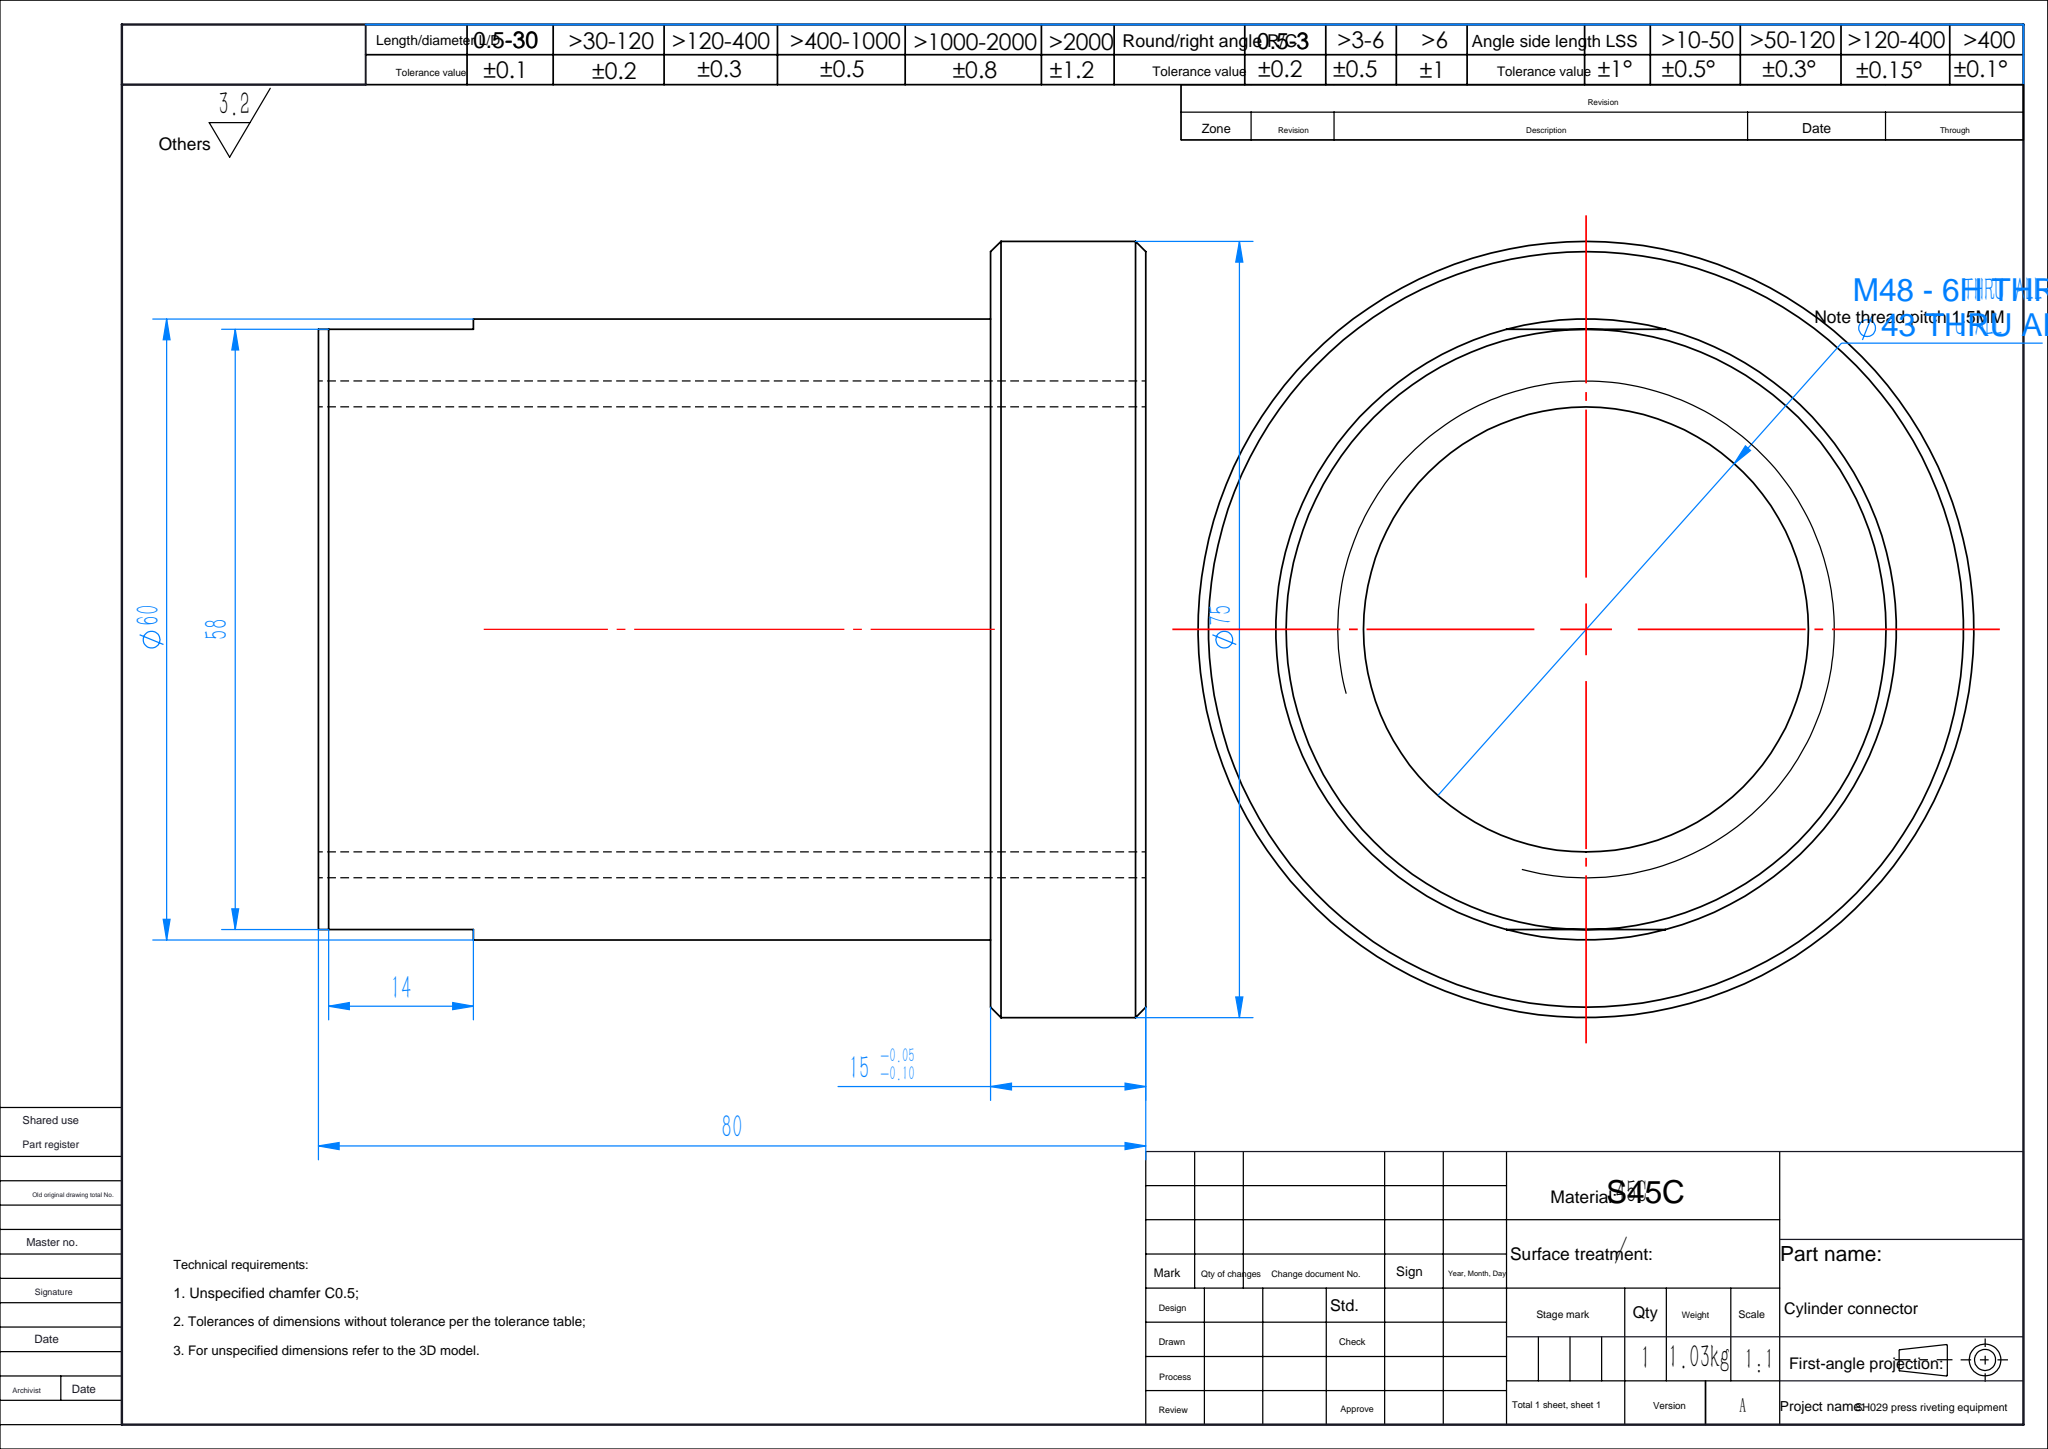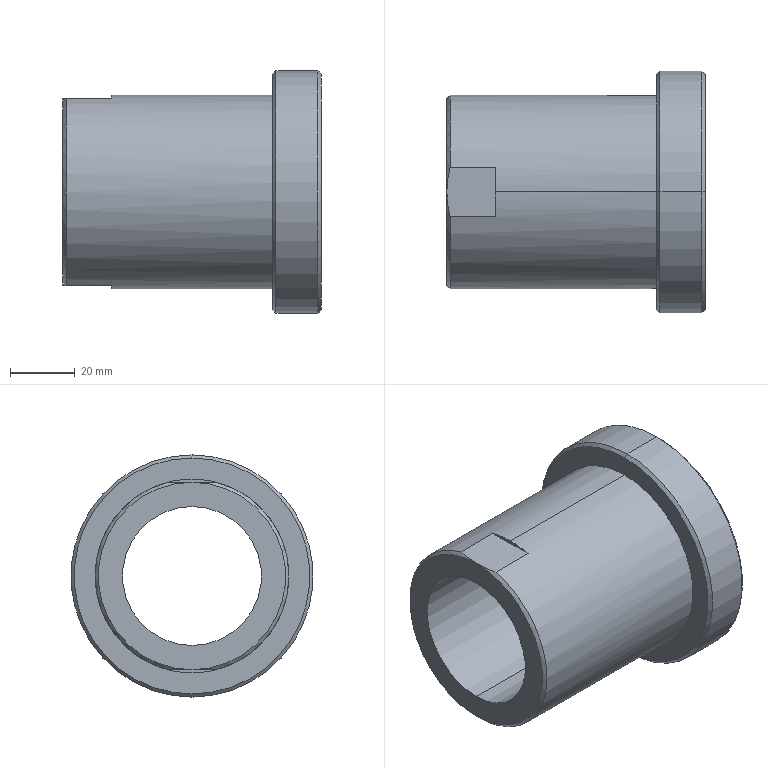Part | SolidWorks | features Chamfer 1, HoleWzd 1, ICE 1, LibraryFeature 1, Revolution 1 | 1 solid | 19 faces | box 80 x 75 x 75 mm | volume 133252 mm3 | plane 7 | cone 6 | cylinder 6 | commonest cylinder face diameters 43 x2 60 x2 75 x2
STEP:
#1=CARTESIAN_POINT('',(25.,0.,36.5));
#2=VERTEX_POINT('',#1);
#3=CARTESIAN_POINT('',(25.,0.,-36.5));
#4=VERTEX_POINT('',#3);
#5=CARTESIAN_POINT('',(25.,0.,0.));
#6=DIRECTION('',(-1.,0.,0.));
#7=DIRECTION('',(0.,0.,-1.));
#8=AXIS2_PLACEMENT_3D('',#5,#6,#7);
#9=CIRCLE('',#8,36.5);
#10=EDGE_CURVE('',#2,#4,#9,.T.);
#11=ORIENTED_EDGE('',*,*,#10,.F.);
#12=CARTESIAN_POINT('',(26.,0.,37.5));
#13=VERTEX_POINT('',#12);
#14=CARTESIAN_POINT('',(25.,0.,36.5));
#15=DIRECTION('',(0.7071,0.,0.7071));
#16=VECTOR('',#15,1000.);
#17=LINE('',#14,#16);
#18=EDGE_CURVE('',#2,#13,#17,.T.);
#19=ORIENTED_EDGE('',*,*,#18,.T.);
#20=CARTESIAN_POINT('',(26.,0.,-37.5));
#21=VERTEX_POINT('',#20);
#22=CARTESIAN_POINT('',(26.,0.,0.));
#23=DIRECTION('',(1.,0.,0.));
#24=DIRECTION('',(0.,0.,-1.));
#25=AXIS2_PLACEMENT_3D('',#22,#23,#24);
#26=CIRCLE('',#25,37.5);
#27=EDGE_CURVE('',#21,#13,#26,.T.);
#28=ORIENTED_EDGE('',*,*,#27,.F.);
#29=CARTESIAN_POINT('',(25.,0.,-36.5));
#30=DIRECTION('',(0.7071,0.,-0.7071));
#31=VECTOR('',#30,1000.);
#32=LINE('',#29,#31);
#33=EDGE_CURVE('',#4,#21,#32,.T.);
#34=ORIENTED_EDGE('',*,*,#33,.F.);
#35=EDGE_LOOP('',(#11,#19,#28,#34));
#36=FACE_OUTER_BOUND('',#35,.T.);
#37=CARTESIAN_POINT('',(25.,0.,0.));
#38=DIRECTION('',(1.,0.,0.));
#39=DIRECTION('',(0.,0.,-1.));
#40=AXIS2_PLACEMENT_3D('',#37,#38,#39);
#41=CONICAL_SURFACE('',#40,36.5,0.7854);
#42=ADVANCED_FACE('',(#36),#41,.T.);
#43=CARTESIAN_POINT('',(40.,0.,-36.5));
#44=VERTEX_POINT('',#43);
#45=CARTESIAN_POINT('',(40.,0.,36.5));
#46=VERTEX_POINT('',#45);
#47=CARTESIAN_POINT('',(40.,0.,0.));
#48=DIRECTION('',(1.,0.,0.));
#49=DIRECTION('',(0.,0.,1.));
#50=AXIS2_PLACEMENT_3D('',#47,#48,#49);
#51=CIRCLE('',#50,36.5);
#52=EDGE_CURVE('',#44,#46,#51,.T.);
#53=ORIENTED_EDGE('',*,*,#52,.F.);
#54=CARTESIAN_POINT('',(39.,0.,-37.5));
#55=VERTEX_POINT('',#54);
#56=CARTESIAN_POINT('',(39.,0.,-37.5));
#57=DIRECTION('',(-0.7071,0.,-0.7071));
#58=VECTOR('',#57,1000.);
#59=LINE('',#56,#58);
#60=EDGE_CURVE('',#44,#55,#59,.T.);
#61=ORIENTED_EDGE('',*,*,#60,.T.);
#62=CARTESIAN_POINT('',(39.,0.,37.5));
#63=VERTEX_POINT('',#62);
#64=CARTESIAN_POINT('',(39.,0.,0.));
#65=DIRECTION('',(-1.,0.,0.));
#66=DIRECTION('',(0.,0.,1.));
#67=AXIS2_PLACEMENT_3D('',#64,#65,#66);
#68=CIRCLE('',#67,37.5);
#69=EDGE_CURVE('',#63,#55,#68,.T.);
#70=ORIENTED_EDGE('',*,*,#69,.F.);
#71=CARTESIAN_POINT('',(39.,0.,37.5));
#72=DIRECTION('',(-0.7071,0.,0.7071));
#73=VECTOR('',#72,1000.);
#74=LINE('',#71,#73);
#75=EDGE_CURVE('',#46,#63,#74,.T.);
#76=ORIENTED_EDGE('',*,*,#75,.F.);
#77=EDGE_LOOP('',(#53,#61,#70,#76));
#78=FACE_OUTER_BOUND('',#77,.T.);
#79=CARTESIAN_POINT('',(39.,0.,0.));
#80=DIRECTION('',(-1.,0.,0.));
#81=DIRECTION('',(0.,0.,1.));
#82=AXIS2_PLACEMENT_3D('',#79,#80,#81);
#83=CONICAL_SURFACE('',#82,37.5,0.7854);
#84=ADVANCED_FACE('',(#78),#83,.T.);
#85=CARTESIAN_POINT('',(40.,0.,-21.5));
#86=VERTEX_POINT('',#85);
#87=CARTESIAN_POINT('',(40.,0.,21.5));
#88=VERTEX_POINT('',#87);
#89=CARTESIAN_POINT('',(40.,0.,0.));
#90=DIRECTION('',(-1.,0.,0.));
#91=DIRECTION('',(0.,0.,1.));
#92=AXIS2_PLACEMENT_3D('',#89,#90,#91);
#93=CIRCLE('',#92,21.5);
#94=EDGE_CURVE('',#86,#88,#93,.T.);
#95=ORIENTED_EDGE('',*,*,#94,.F.);
#96=CARTESIAN_POINT('',(-40.,0.,-21.5));
#97=VERTEX_POINT('',#96);
#98=CARTESIAN_POINT('',(-40.,0.,-21.5));
#99=DIRECTION('',(-1.,0.,0.));
#100=VECTOR('',#99,1000.);
#101=LINE('',#98,#100);
#102=EDGE_CURVE('',#86,#97,#101,.T.);
#103=ORIENTED_EDGE('',*,*,#102,.T.);
#104=CARTESIAN_POINT('',(-40.,0.,21.5));
#105=VERTEX_POINT('',#104);
#106=CARTESIAN_POINT('',(-40.,0.,0.));
#107=DIRECTION('',(-1.,0.,0.));
#108=DIRECTION('',(0.,0.,1.));
#109=AXIS2_PLACEMENT_3D('',#106,#107,#108);
#110=CIRCLE('',#109,21.5);
#111=EDGE_CURVE('',#97,#105,#110,.T.);
#112=ORIENTED_EDGE('',*,*,#111,.T.);
#113=CARTESIAN_POINT('',(-40.,0.,21.5));
#114=DIRECTION('',(-1.,0.,0.));
#115=VECTOR('',#114,1000.);
#116=LINE('',#113,#115);
#117=EDGE_CURVE('',#88,#105,#116,.T.);
#118=ORIENTED_EDGE('',*,*,#117,.F.);
#119=EDGE_LOOP('',(#95,#103,#112,#118));
#120=FACE_OUTER_BOUND('',#119,.T.);
#121=CARTESIAN_POINT('',(-40.,0.,0.));
#122=DIRECTION('',(-1.,0.,0.));
#123=DIRECTION('',(0.,0.,1.));
#124=AXIS2_PLACEMENT_3D('',#121,#122,#123);
#125=CYLINDRICAL_SURFACE('',#124,21.5);
#126=ADVANCED_FACE('',(#120),#125,.F.);
#127=ORIENTED_EDGE('',*,*,#69,.T.);
#128=CARTESIAN_POINT('',(-111.455,0.,-37.5));
#129=DIRECTION('',(-1.,0.,0.));
#130=VECTOR('',#129,1000.);
#131=LINE('',#128,#130);
#132=EDGE_CURVE('',#55,#21,#131,.T.);
#133=ORIENTED_EDGE('',*,*,#132,.T.);
#134=ORIENTED_EDGE('',*,*,#27,.T.);
#135=CARTESIAN_POINT('',(-111.455,0.,37.5));
#136=DIRECTION('',(-1.,0.,0.));
#137=VECTOR('',#136,1000.);
#138=LINE('',#135,#137);
#139=EDGE_CURVE('',#63,#13,#138,.T.);
#140=ORIENTED_EDGE('',*,*,#139,.F.);
#141=EDGE_LOOP('',(#127,#133,#134,#140));
#142=FACE_OUTER_BOUND('',#141,.T.);
#143=CARTESIAN_POINT('',(-111.455,0.,0.));
#144=DIRECTION('',(-1.,0.,0.));
#145=DIRECTION('',(0.,0.,1.));
#146=AXIS2_PLACEMENT_3D('',#143,#144,#145);
#147=CYLINDRICAL_SURFACE('',#146,37.5);
#148=ADVANCED_FACE('',(#142),#147,.T.);
#149=CARTESIAN_POINT('',(25.,0.,30.));
#150=VERTEX_POINT('',#149);
#151=CARTESIAN_POINT('',(25.,0.,-30.));
#152=VERTEX_POINT('',#151);
#153=CARTESIAN_POINT('',(25.,0.,0.));
#154=DIRECTION('',(-1.,0.,0.));
#155=DIRECTION('',(0.,0.,1.));
#156=AXIS2_PLACEMENT_3D('',#153,#154,#155);
#157=CIRCLE('',#156,30.);
#158=EDGE_CURVE('',#150,#152,#157,.T.);
#159=ORIENTED_EDGE('',*,*,#158,.T.);
#160=CARTESIAN_POINT('',(-25.,0.,-30.));
#161=VERTEX_POINT('',#160);
#162=CARTESIAN_POINT('',(-111.455,0.,-30.));
#163=DIRECTION('',(-1.,0.,0.));
#164=VECTOR('',#163,1000.);
#165=LINE('',#162,#164);
#166=EDGE_CURVE('',#152,#161,#165,.T.);
#167=ORIENTED_EDGE('',*,*,#166,.T.);
#168=CARTESIAN_POINT('',(-25.,7.681,-29.));
#169=VERTEX_POINT('',#168);
#170=CARTESIAN_POINT('',(-25.,0.,0.));
#171=DIRECTION('',(1.,0.,0.));
#172=DIRECTION('',(0.,0.,-1.));
#173=AXIS2_PLACEMENT_3D('',#170,#171,#172);
#174=CIRCLE('',#173,30.);
#175=EDGE_CURVE('',#161,#169,#174,.T.);
#176=ORIENTED_EDGE('',*,*,#175,.T.);
#177=CARTESIAN_POINT('',(-39.,7.681,-29.));
#178=VERTEX_POINT('',#177);
#179=CARTESIAN_POINT('',(-111.455,7.681,-29.));
#180=DIRECTION('',(-1.,0.,0.));
#181=VECTOR('',#180,1000.);
#182=LINE('',#179,#181);
#183=EDGE_CURVE('',#169,#178,#182,.T.);
#184=ORIENTED_EDGE('',*,*,#183,.T.);
#185=CARTESIAN_POINT('',(-39.,7.681,29.));
#186=VERTEX_POINT('',#185);
#187=CARTESIAN_POINT('',(-39.,0.,0.));
#188=DIRECTION('',(1.,0.,0.));
#189=DIRECTION('',(0.,0.,-1.));
#190=AXIS2_PLACEMENT_3D('',#187,#188,#189);
#191=CIRCLE('',#190,30.);
#192=EDGE_CURVE('',#178,#186,#191,.T.);
#193=ORIENTED_EDGE('',*,*,#192,.T.);
#194=CARTESIAN_POINT('',(-25.,7.681,29.));
#195=VERTEX_POINT('',#194);
#196=CARTESIAN_POINT('',(-111.455,7.681,29.));
#197=DIRECTION('',(1.,0.,0.));
#198=VECTOR('',#197,1000.);
#199=LINE('',#196,#198);
#200=EDGE_CURVE('',#186,#195,#199,.T.);
#201=ORIENTED_EDGE('',*,*,#200,.T.);
#202=CARTESIAN_POINT('',(-25.,0.,30.));
#203=VERTEX_POINT('',#202);
#204=CARTESIAN_POINT('',(-25.,0.,0.));
#205=DIRECTION('',(-1.,0.,0.));
#206=DIRECTION('',(0.,0.,1.));
#207=AXIS2_PLACEMENT_3D('',#204,#205,#206);
#208=CIRCLE('',#207,30.);
#209=EDGE_CURVE('',#203,#195,#208,.T.);
#210=ORIENTED_EDGE('',*,*,#209,.F.);
#211=CARTESIAN_POINT('',(-111.455,0.,30.));
#212=DIRECTION('',(-1.,0.,0.));
#213=VECTOR('',#212,1000.);
#214=LINE('',#211,#213);
#215=EDGE_CURVE('',#150,#203,#214,.T.);
#216=ORIENTED_EDGE('',*,*,#215,.F.);
#217=EDGE_LOOP('',(#159,#167,#176,#184,#193,#201,#210,#216));
#218=FACE_OUTER_BOUND('',#217,.T.);
#219=CARTESIAN_POINT('',(-111.455,0.,0.));
#220=DIRECTION('',(-1.,0.,0.));
#221=DIRECTION('',(0.,0.,1.));
#222=AXIS2_PLACEMENT_3D('',#219,#220,#221);
#223=CYLINDRICAL_SURFACE('',#222,30.);
#224=ADVANCED_FACE('',(#218),#223,.T.);
#225=CARTESIAN_POINT('',(-40.,0.,0.));
#226=DIRECTION('',(-1.,0.,0.));
#227=DIRECTION('',(0.,0.,1.));
#228=AXIS2_PLACEMENT_3D('',#225,#226,#227);
#229=CIRCLE('',#228,21.5);
#230=EDGE_CURVE('',#105,#97,#229,.T.);
#231=ORIENTED_EDGE('',*,*,#230,.F.);
#232=ORIENTED_EDGE('',*,*,#111,.F.);
#233=EDGE_LOOP('',(#231,#232));
#234=FACE_BOUND('',#233,.T.);
#235=CARTESIAN_POINT('',(-40.,0.,29.));
#236=VERTEX_POINT('',#235);
#237=CARTESIAN_POINT('',(-40.,0.,-29.));
#238=VERTEX_POINT('',#237);
#239=CARTESIAN_POINT('',(-40.,0.,0.));
#240=DIRECTION('',(-1.,0.,0.));
#241=DIRECTION('',(0.,0.,-1.));
#242=AXIS2_PLACEMENT_3D('',#239,#240,#241);
#243=CIRCLE('',#242,29.);
#244=EDGE_CURVE('',#236,#238,#243,.T.);
#245=ORIENTED_EDGE('',*,*,#244,.T.);
#246=CARTESIAN_POINT('',(-40.,0.,0.));
#247=DIRECTION('',(-1.,0.,0.));
#248=DIRECTION('',(0.,0.,-1.));
#249=AXIS2_PLACEMENT_3D('',#246,#247,#248);
#250=CIRCLE('',#249,29.);
#251=EDGE_CURVE('',#238,#236,#250,.T.);
#252=ORIENTED_EDGE('',*,*,#251,.T.);
#253=EDGE_LOOP('',(#245,#252));
#254=FACE_OUTER_BOUND('',#253,.T.);
#255=CARTESIAN_POINT('',(-40.,0.,0.));
#256=DIRECTION('',(1.,0.,0.));
#257=DIRECTION('',(0.,0.,-1.));
#258=AXIS2_PLACEMENT_3D('',#255,#256,#257);
#259=PLANE('',#258);
#260=ADVANCED_FACE('',(#234,#254),#259,.F.);
#261=ORIENTED_EDGE('',*,*,#166,.F.);
#262=CARTESIAN_POINT('',(25.,0.,0.));
#263=DIRECTION('',(-1.,0.,0.));
#264=DIRECTION('',(0.,0.,1.));
#265=AXIS2_PLACEMENT_3D('',#262,#263,#264);
#266=CIRCLE('',#265,30.);
#267=EDGE_CURVE('',#152,#150,#266,.T.);
#268=ORIENTED_EDGE('',*,*,#267,.T.);
#269=ORIENTED_EDGE('',*,*,#215,.T.);
#270=CARTESIAN_POINT('',(-25.,-7.681,29.));
#271=VERTEX_POINT('',#270);
#272=CARTESIAN_POINT('',(-25.,0.,0.));
#273=DIRECTION('',(-1.,0.,0.));
#274=DIRECTION('',(0.,0.,1.));
#275=AXIS2_PLACEMENT_3D('',#272,#273,#274);
#276=CIRCLE('',#275,30.);
#277=EDGE_CURVE('',#271,#203,#276,.T.);
#278=ORIENTED_EDGE('',*,*,#277,.F.);
#279=CARTESIAN_POINT('',(-39.,-7.681,29.));
#280=VERTEX_POINT('',#279);
#281=CARTESIAN_POINT('',(-111.455,-7.681,29.));
#282=DIRECTION('',(-1.,0.,0.));
#283=VECTOR('',#282,1000.);
#284=LINE('',#281,#283);
#285=EDGE_CURVE('',#271,#280,#284,.T.);
#286=ORIENTED_EDGE('',*,*,#285,.T.);
#287=CARTESIAN_POINT('',(-39.,-7.681,-29.));
#288=VERTEX_POINT('',#287);
#289=CARTESIAN_POINT('',(-39.,0.,0.));
#290=DIRECTION('',(1.,0.,0.));
#291=DIRECTION('',(0.,0.,-1.));
#292=AXIS2_PLACEMENT_3D('',#289,#290,#291);
#293=CIRCLE('',#292,30.);
#294=EDGE_CURVE('',#280,#288,#293,.T.);
#295=ORIENTED_EDGE('',*,*,#294,.T.);
#296=CARTESIAN_POINT('',(-25.,-7.681,-29.));
#297=VERTEX_POINT('',#296);
#298=CARTESIAN_POINT('',(-111.455,-7.681,-29.));
#299=DIRECTION('',(1.,0.,0.));
#300=VECTOR('',#299,1000.);
#301=LINE('',#298,#300);
#302=EDGE_CURVE('',#288,#297,#301,.T.);
#303=ORIENTED_EDGE('',*,*,#302,.T.);
#304=CARTESIAN_POINT('',(-25.,0.,0.));
#305=DIRECTION('',(1.,0.,0.));
#306=DIRECTION('',(0.,0.,-1.));
#307=AXIS2_PLACEMENT_3D('',#304,#305,#306);
#308=CIRCLE('',#307,30.);
#309=EDGE_CURVE('',#297,#161,#308,.T.);
#310=ORIENTED_EDGE('',*,*,#309,.T.);
#311=EDGE_LOOP('',(#261,#268,#269,#278,#286,#295,#303,#310));
#312=FACE_OUTER_BOUND('',#311,.T.);
#313=CARTESIAN_POINT('',(-111.455,0.,0.));
#314=DIRECTION('',(-1.,0.,0.));
#315=DIRECTION('',(0.,0.,1.));
#316=AXIS2_PLACEMENT_3D('',#313,#314,#315);
#317=CYLINDRICAL_SURFACE('',#316,30.);
#318=ADVANCED_FACE('',(#312),#317,.T.);
#319=CARTESIAN_POINT('',(25.,0.,0.));
#320=DIRECTION('',(-1.,0.,0.));
#321=DIRECTION('',(0.,0.,-1.));
#322=AXIS2_PLACEMENT_3D('',#319,#320,#321);
#323=CIRCLE('',#322,36.5);
#324=EDGE_CURVE('',#4,#2,#323,.T.);
#325=ORIENTED_EDGE('',*,*,#324,.T.);
#326=ORIENTED_EDGE('',*,*,#10,.T.);
#327=EDGE_LOOP('',(#325,#326));
#328=FACE_OUTER_BOUND('',#327,.T.);
#329=ORIENTED_EDGE('',*,*,#158,.F.);
#330=ORIENTED_EDGE('',*,*,#267,.F.);
#331=EDGE_LOOP('',(#329,#330));
#332=FACE_BOUND('',#331,.T.);
#333=CARTESIAN_POINT('',(25.,0.,-30.));
#334=DIRECTION('',(1.,0.,0.));
#335=DIRECTION('',(0.,0.,-1.));
#336=AXIS2_PLACEMENT_3D('',#333,#334,#335);
#337=PLANE('',#336);
#338=ADVANCED_FACE('',(#328,#332),#337,.F.);
#339=ORIENTED_EDGE('',*,*,#132,.F.);
#340=CARTESIAN_POINT('',(39.,0.,0.));
#341=DIRECTION('',(-1.,0.,0.));
#342=DIRECTION('',(0.,0.,1.));
#343=AXIS2_PLACEMENT_3D('',#340,#341,#342);
#344=CIRCLE('',#343,37.5);
#345=EDGE_CURVE('',#55,#63,#344,.T.);
#346=ORIENTED_EDGE('',*,*,#345,.T.);
#347=ORIENTED_EDGE('',*,*,#139,.T.);
#348=CARTESIAN_POINT('',(26.,0.,0.));
#349=DIRECTION('',(1.,0.,0.));
#350=DIRECTION('',(0.,0.,-1.));
#351=AXIS2_PLACEMENT_3D('',#348,#349,#350);
#352=CIRCLE('',#351,37.5);
#353=EDGE_CURVE('',#13,#21,#352,.T.);
#354=ORIENTED_EDGE('',*,*,#353,.T.);
#355=EDGE_LOOP('',(#339,#346,#347,#354));
#356=FACE_OUTER_BOUND('',#355,.T.);
#357=CARTESIAN_POINT('',(-111.455,0.,0.));
#358=DIRECTION('',(-1.,0.,0.));
#359=DIRECTION('',(0.,0.,1.));
#360=AXIS2_PLACEMENT_3D('',#357,#358,#359);
#361=CYLINDRICAL_SURFACE('',#360,37.5);
#362=ADVANCED_FACE('',(#356),#361,.T.);
#363=CARTESIAN_POINT('',(40.,0.,0.));
#364=DIRECTION('',(1.,0.,0.));
#365=DIRECTION('',(0.,0.,1.));
#366=AXIS2_PLACEMENT_3D('',#363,#364,#365);
#367=CIRCLE('',#366,36.5);
#368=EDGE_CURVE('',#46,#44,#367,.T.);
#369=ORIENTED_EDGE('',*,*,#368,.T.);
#370=ORIENTED_EDGE('',*,*,#52,.T.);
#371=EDGE_LOOP('',(#369,#370));
#372=FACE_OUTER_BOUND('',#371,.T.);
#373=CARTESIAN_POINT('',(40.,0.,0.));
#374=DIRECTION('',(-1.,0.,0.));
#375=DIRECTION('',(0.,0.,1.));
#376=AXIS2_PLACEMENT_3D('',#373,#374,#375);
#377=CIRCLE('',#376,21.5);
#378=EDGE_CURVE('',#88,#86,#377,.T.);
#379=ORIENTED_EDGE('',*,*,#378,.T.);
#380=ORIENTED_EDGE('',*,*,#94,.T.);
#381=EDGE_LOOP('',(#379,#380));
#382=FACE_BOUND('',#381,.T.);
#383=CARTESIAN_POINT('',(40.,0.,-37.5));
#384=DIRECTION('',(-1.,0.,0.));
#385=DIRECTION('',(0.,0.,1.));
#386=AXIS2_PLACEMENT_3D('',#383,#384,#385);
#387=PLANE('',#386);
#388=ADVANCED_FACE('',(#372,#382),#387,.F.);
#389=ORIENTED_EDGE('',*,*,#102,.F.);
#390=ORIENTED_EDGE('',*,*,#378,.F.);
#391=ORIENTED_EDGE('',*,*,#117,.T.);
#392=ORIENTED_EDGE('',*,*,#230,.T.);
#393=EDGE_LOOP('',(#389,#390,#391,#392));
#394=FACE_OUTER_BOUND('',#393,.T.);
#395=CARTESIAN_POINT('',(-40.,0.,0.));
#396=DIRECTION('',(-1.,0.,0.));
#397=DIRECTION('',(0.,0.,1.));
#398=AXIS2_PLACEMENT_3D('',#395,#396,#397);
#399=CYLINDRICAL_SURFACE('',#398,21.5);
#400=ADVANCED_FACE('',(#394),#399,.F.);
#401=CARTESIAN_POINT('',(-39.,7.681,29.));
#402=CARTESIAN_POINT('',(-39.645,5.161,29.));
#403=CARTESIAN_POINT('',(-40.,2.604,29.));
#404=CARTESIAN_POINT('',(-40.,0.,29.));
#405=B_SPLINE_CURVE_WITH_KNOTS('',3,(#401,#402,#403,#404),.UNSPECIFIED.,.F.,.F.,(4,4),(0.,0.007746),.UNSPECIFIED.);
#406=EDGE_CURVE('',#186,#236,#405,.T.);
#407=ORIENTED_EDGE('',*,*,#406,.T.);
#408=CARTESIAN_POINT('',(-40.,0.,29.));
#409=CARTESIAN_POINT('',(-40.,-2.604,29.));
#410=CARTESIAN_POINT('',(-39.645,-5.161,29.));
#411=CARTESIAN_POINT('',(-39.,-7.681,29.));
#412=B_SPLINE_CURVE_WITH_KNOTS('',3,(#408,#409,#410,#411),.UNSPECIFIED.,.F.,.F.,(4,4),(0.,0.007746),.UNSPECIFIED.);
#413=EDGE_CURVE('',#236,#280,#412,.T.);
#414=ORIENTED_EDGE('',*,*,#413,.T.);
#415=ORIENTED_EDGE('',*,*,#285,.F.);
#416=CARTESIAN_POINT('',(-25.,30.,29.));
#417=DIRECTION('',(0.,-1.,0.));
#418=VECTOR('',#417,1000.);
#419=LINE('',#416,#418);
#420=EDGE_CURVE('',#195,#271,#419,.T.);
#421=ORIENTED_EDGE('',*,*,#420,.F.);
#422=ORIENTED_EDGE('',*,*,#200,.F.);
#423=EDGE_LOOP('',(#407,#414,#415,#421,#422));
#424=FACE_OUTER_BOUND('',#423,.T.);
#425=CARTESIAN_POINT('',(-25.,30.,29.));
#426=DIRECTION('',(0.,0.,-1.));
#427=DIRECTION('',(0.,1.,0.));
#428=AXIS2_PLACEMENT_3D('',#425,#426,#427);
#429=PLANE('',#428);
#430=ADVANCED_FACE('',(#424),#429,.F.);
#431=ORIENTED_EDGE('',*,*,#277,.T.);
#432=ORIENTED_EDGE('',*,*,#209,.T.);
#433=ORIENTED_EDGE('',*,*,#420,.T.);
#434=EDGE_LOOP('',(#431,#432,#433));
#435=FACE_OUTER_BOUND('',#434,.T.);
#436=CARTESIAN_POINT('',(-25.,0.,0.));
#437=DIRECTION('',(-1.,0.,0.));
#438=DIRECTION('',(0.,0.,1.));
#439=AXIS2_PLACEMENT_3D('',#436,#437,#438);
#440=PLANE('',#439);
#441=ADVANCED_FACE('',(#435),#440,.T.);
#442=ORIENTED_EDGE('',*,*,#302,.F.);
#443=CARTESIAN_POINT('',(-39.,-7.681,-29.));
#444=CARTESIAN_POINT('',(-39.645,-5.161,-29.));
#445=CARTESIAN_POINT('',(-40.,-2.604,-29.));
#446=CARTESIAN_POINT('',(-40.,0.,-29.));
#447=B_SPLINE_CURVE_WITH_KNOTS('',3,(#443,#444,#445,#446),.UNSPECIFIED.,.F.,.F.,(4,4),(0.,0.007746),.UNSPECIFIED.);
#448=EDGE_CURVE('',#288,#238,#447,.T.);
#449=ORIENTED_EDGE('',*,*,#448,.T.);
#450=CARTESIAN_POINT('',(-40.,0.,-29.));
#451=CARTESIAN_POINT('',(-40.,2.604,-29.));
#452=CARTESIAN_POINT('',(-39.645,5.161,-29.));
#453=CARTESIAN_POINT('',(-39.,7.681,-29.));
#454=B_SPLINE_CURVE_WITH_KNOTS('',3,(#450,#451,#452,#453),.UNSPECIFIED.,.F.,.F.,(4,4),(0.,0.007746),.UNSPECIFIED.);
#455=EDGE_CURVE('',#238,#178,#454,.T.);
#456=ORIENTED_EDGE('',*,*,#455,.T.);
#457=ORIENTED_EDGE('',*,*,#183,.F.);
#458=CARTESIAN_POINT('',(-25.,30.,-29.));
#459=DIRECTION('',(0.,1.,0.));
#460=VECTOR('',#459,1000.);
#461=LINE('',#458,#460);
#462=EDGE_CURVE('',#297,#169,#461,.T.);
#463=ORIENTED_EDGE('',*,*,#462,.F.);
#464=EDGE_LOOP('',(#442,#449,#456,#457,#463));
#465=FACE_OUTER_BOUND('',#464,.T.);
#466=CARTESIAN_POINT('',(-25.,30.,-29.));
#467=DIRECTION('',(0.,0.,1.));
#468=DIRECTION('',(0.,-1.,0.));
#469=AXIS2_PLACEMENT_3D('',#466,#467,#468);
#470=PLANE('',#469);
#471=ADVANCED_FACE('',(#465),#470,.F.);
#472=ORIENTED_EDGE('',*,*,#309,.F.);
#473=ORIENTED_EDGE('',*,*,#462,.T.);
#474=ORIENTED_EDGE('',*,*,#175,.F.);
#475=EDGE_LOOP('',(#472,#473,#474));
#476=FACE_OUTER_BOUND('',#475,.T.);
#477=CARTESIAN_POINT('',(-25.,0.,0.));
#478=DIRECTION('',(1.,0.,0.));
#479=DIRECTION('',(0.,0.,-1.));
#480=AXIS2_PLACEMENT_3D('',#477,#478,#479);
#481=PLANE('',#480);
#482=ADVANCED_FACE('',(#476),#481,.F.);
#483=ORIENTED_EDGE('',*,*,#60,.F.);
#484=ORIENTED_EDGE('',*,*,#368,.F.);
#485=ORIENTED_EDGE('',*,*,#75,.T.);
#486=ORIENTED_EDGE('',*,*,#345,.F.);
#487=EDGE_LOOP('',(#483,#484,#485,#486));
#488=FACE_OUTER_BOUND('',#487,.T.);
#489=CARTESIAN_POINT('',(39.,0.,0.));
#490=DIRECTION('',(-1.,0.,0.));
#491=DIRECTION('',(0.,0.,1.));
#492=AXIS2_PLACEMENT_3D('',#489,#490,#491);
#493=CONICAL_SURFACE('',#492,37.5,0.7854);
#494=ADVANCED_FACE('',(#488),#493,.T.);
#495=ORIENTED_EDGE('',*,*,#18,.F.);
#496=ORIENTED_EDGE('',*,*,#324,.F.);
#497=ORIENTED_EDGE('',*,*,#33,.T.);
#498=ORIENTED_EDGE('',*,*,#353,.F.);
#499=EDGE_LOOP('',(#495,#496,#497,#498));
#500=FACE_OUTER_BOUND('',#499,.T.);
#501=CARTESIAN_POINT('',(25.,0.,0.));
#502=DIRECTION('',(1.,0.,0.));
#503=DIRECTION('',(0.,0.,-1.));
#504=AXIS2_PLACEMENT_3D('',#501,#502,#503);
#505=CONICAL_SURFACE('',#504,36.5,0.7854);
#506=ADVANCED_FACE('',(#500),#505,.T.);
#507=ORIENTED_EDGE('',*,*,#448,.F.);
#508=ORIENTED_EDGE('',*,*,#294,.F.);
#509=ORIENTED_EDGE('',*,*,#413,.F.);
#510=ORIENTED_EDGE('',*,*,#251,.F.);
#511=EDGE_LOOP('',(#507,#508,#509,#510));
#512=FACE_OUTER_BOUND('',#511,.T.);
#513=CARTESIAN_POINT('',(-40.,0.,0.));
#514=DIRECTION('',(1.,0.,0.));
#515=DIRECTION('',(0.,0.,-1.));
#516=AXIS2_PLACEMENT_3D('',#513,#514,#515);
#517=CONICAL_SURFACE('',#516,29.,0.7854);
#518=ADVANCED_FACE('',(#512),#517,.T.);
#519=ORIENTED_EDGE('',*,*,#406,.F.);
#520=ORIENTED_EDGE('',*,*,#192,.F.);
#521=ORIENTED_EDGE('',*,*,#455,.F.);
#522=ORIENTED_EDGE('',*,*,#244,.F.);
#523=EDGE_LOOP('',(#519,#520,#521,#522));
#524=FACE_OUTER_BOUND('',#523,.T.);
#525=CARTESIAN_POINT('',(-40.,0.,0.));
#526=DIRECTION('',(1.,0.,0.));
#527=DIRECTION('',(0.,0.,-1.));
#528=AXIS2_PLACEMENT_3D('',#525,#526,#527);
#529=CONICAL_SURFACE('',#528,29.,0.7854);
#530=ADVANCED_FACE('',(#524),#529,.T.);
#531=CLOSED_SHELL('',(#42,#84,#126,#148,#224,#260,#318,#338,#362,#388,#400,#430,#441,#471,#482,#494,#506,#518,#530));
#532=MANIFOLD_SOLID_BREP('',#531);
#533=CARTESIAN_POINT('',(0.,0.,0.));
#534=DIRECTION('',(0.,0.,1.));
#535=DIRECTION('',(1.,0.,0.));
#536=AXIS2_PLACEMENT_3D('',#533,#534,#535);
#537=(LENGTH_UNIT()NAMED_UNIT(*)SI_UNIT(.MILLI.,.METRE.));
#538=UNCERTAINTY_MEASURE_WITH_UNIT(LENGTH_MEASURE(0.00001),#537,'','');
#539=(NAMED_UNIT(*)PLANE_ANGLE_UNIT()SI_UNIT($,.RADIAN.));
#540=(NAMED_UNIT(*)SI_UNIT($,.STERADIAN.)SOLID_ANGLE_UNIT());
#541=(GEOMETRIC_REPRESENTATION_CONTEXT(3)GLOBAL_UNCERTAINTY_ASSIGNED_CONTEXT((#538))GLOBAL_UNIT_ASSIGNED_CONTEXT((#537,#539,#540))REPRESENTATION_CONTEXT('',''));
#542=ADVANCED_BREP_SHAPE_REPRESENTATION('',(#532,#536),#541);